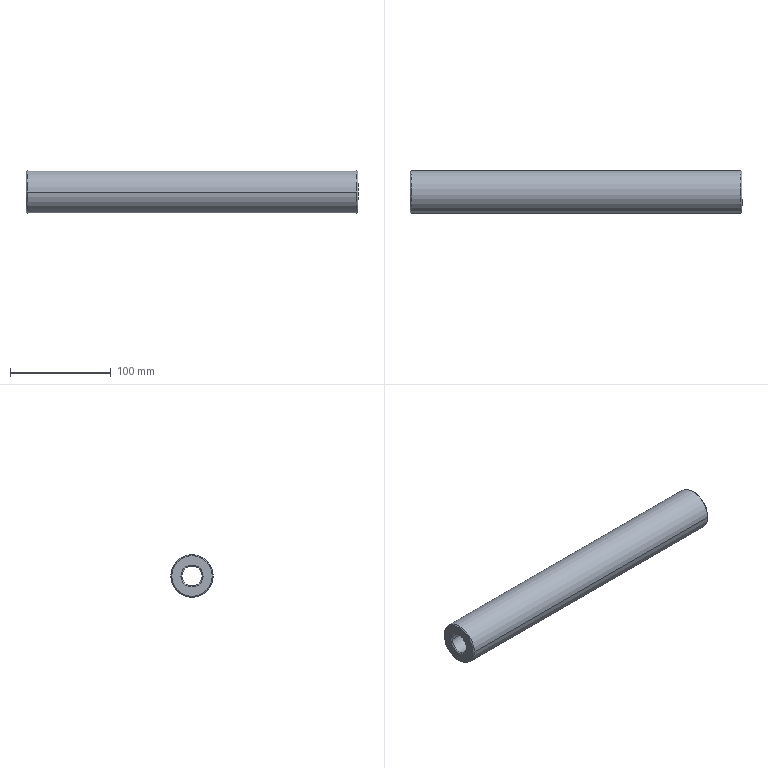Part | SolidWorks | features BaseBody 1 | 1 solid | 20 faces | box 330 x 42.2 x 42.2 mm | volume 188080 mm3 | cylinder 8 | cone 8 | plane 4 | commonest cylinder face diameters 20 x4 35.08 x2 42.2 x2
STEP:
#1=CARTESIAN_POINT('',(-40.109,46.064,0.));
#2=VERTEX_POINT('',#1);
#3=CARTESIAN_POINT('',(-40.109,3.864,0.));
#4=VERTEX_POINT('',#3);
#5=CARTESIAN_POINT('',(-40.109,24.964,0.));
#6=DIRECTION('',(1.,0.,0.));
#7=DIRECTION('',(0.,1.,0.));
#8=AXIS2_PLACEMENT_3D('',#5,#6,#7);
#9=CIRCLE('',#8,21.1);
#10=EDGE_CURVE('',#2,#4,#9,.T.);
#11=ORIENTED_EDGE('',*,*,#10,.T.);
#12=CARTESIAN_POINT('',(287.891,3.864,0.));
#13=VERTEX_POINT('',#12);
#14=CARTESIAN_POINT('',(123.891,3.864,0.));
#15=DIRECTION('',(1.,0.,0.));
#16=VECTOR('',#15,1000.);
#17=LINE('',#14,#16);
#18=EDGE_CURVE('',#4,#13,#17,.T.);
#19=ORIENTED_EDGE('',*,*,#18,.T.);
#20=CARTESIAN_POINT('',(287.891,46.064,0.));
#21=VERTEX_POINT('',#20);
#22=CARTESIAN_POINT('',(287.891,24.964,0.));
#23=DIRECTION('',(-1.,0.,0.));
#24=DIRECTION('',(0.,1.,0.));
#25=AXIS2_PLACEMENT_3D('',#22,#23,#24);
#26=CIRCLE('',#25,21.1);
#27=EDGE_CURVE('',#13,#21,#26,.T.);
#28=ORIENTED_EDGE('',*,*,#27,.T.);
#29=CARTESIAN_POINT('',(123.891,46.064,0.));
#30=DIRECTION('',(1.,0.,0.));
#31=VECTOR('',#30,1000.);
#32=LINE('',#29,#31);
#33=EDGE_CURVE('',#2,#21,#32,.T.);
#34=ORIENTED_EDGE('',*,*,#33,.F.);
#35=EDGE_LOOP('',(#11,#19,#28,#34));
#36=FACE_OUTER_BOUND('',#35,.T.);
#37=CARTESIAN_POINT('',(123.891,24.964,0.));
#38=DIRECTION('',(1.,0.,0.));
#39=DIRECTION('',(0.,1.,0.));
#40=AXIS2_PLACEMENT_3D('',#37,#38,#39);
#41=CYLINDRICAL_SURFACE('',#40,21.1);
#42=ADVANCED_FACE('',(#36),#41,.T.);
#43=CARTESIAN_POINT('',(288.891,4.864,0.));
#44=VERTEX_POINT('',#43);
#45=CARTESIAN_POINT('',(288.891,45.064,0.));
#46=VERTEX_POINT('',#45);
#47=CARTESIAN_POINT('',(288.891,24.964,0.));
#48=DIRECTION('',(-1.,0.,0.));
#49=DIRECTION('',(0.,-1.,0.));
#50=AXIS2_PLACEMENT_3D('',#47,#48,#49);
#51=CIRCLE('',#50,20.1);
#52=EDGE_CURVE('',#44,#46,#51,.T.);
#53=ORIENTED_EDGE('',*,*,#52,.T.);
#54=CARTESIAN_POINT('',(287.891,46.064,0.));
#55=DIRECTION('',(-0.7071,0.7071,0.));
#56=VECTOR('',#55,1000.);
#57=LINE('',#54,#56);
#58=EDGE_CURVE('',#46,#21,#57,.T.);
#59=ORIENTED_EDGE('',*,*,#58,.T.);
#60=ORIENTED_EDGE('',*,*,#27,.F.);
#61=CARTESIAN_POINT('',(287.891,3.864,0.));
#62=DIRECTION('',(-0.7071,-0.7071,0.));
#63=VECTOR('',#62,1000.);
#64=LINE('',#61,#63);
#65=EDGE_CURVE('',#44,#13,#64,.T.);
#66=ORIENTED_EDGE('',*,*,#65,.F.);
#67=EDGE_LOOP('',(#53,#59,#60,#66));
#68=FACE_OUTER_BOUND('',#67,.T.);
#69=CARTESIAN_POINT('',(287.891,24.964,0.));
#70=DIRECTION('',(-1.,0.,0.));
#71=DIRECTION('',(0.,-1.,0.));
#72=AXIS2_PLACEMENT_3D('',#69,#70,#71);
#73=CONICAL_SURFACE('',#72,21.1,0.7854);
#74=ADVANCED_FACE('',(#68),#73,.T.);
#75=CARTESIAN_POINT('',(-41.109,45.064,0.));
#76=VERTEX_POINT('',#75);
#77=CARTESIAN_POINT('',(-41.109,4.864,0.));
#78=VERTEX_POINT('',#77);
#79=CARTESIAN_POINT('',(-41.109,24.964,0.));
#80=DIRECTION('',(1.,0.,0.));
#81=DIRECTION('',(0.,1.,0.));
#82=AXIS2_PLACEMENT_3D('',#79,#80,#81);
#83=CIRCLE('',#82,20.1);
#84=EDGE_CURVE('',#76,#78,#83,.T.);
#85=ORIENTED_EDGE('',*,*,#84,.T.);
#86=CARTESIAN_POINT('',(-40.109,3.864,0.));
#87=DIRECTION('',(0.7071,-0.7071,0.));
#88=VECTOR('',#87,1000.);
#89=LINE('',#86,#88);
#90=EDGE_CURVE('',#78,#4,#89,.T.);
#91=ORIENTED_EDGE('',*,*,#90,.T.);
#92=ORIENTED_EDGE('',*,*,#10,.F.);
#93=CARTESIAN_POINT('',(-40.109,46.064,0.));
#94=DIRECTION('',(0.7071,0.7071,0.));
#95=VECTOR('',#94,1000.);
#96=LINE('',#93,#95);
#97=EDGE_CURVE('',#76,#2,#96,.T.);
#98=ORIENTED_EDGE('',*,*,#97,.F.);
#99=EDGE_LOOP('',(#85,#91,#92,#98));
#100=FACE_OUTER_BOUND('',#99,.T.);
#101=CARTESIAN_POINT('',(-40.109,24.964,0.));
#102=DIRECTION('',(1.,0.,0.));
#103=DIRECTION('',(0.,1.,0.));
#104=AXIS2_PLACEMENT_3D('',#101,#102,#103);
#105=CONICAL_SURFACE('',#104,21.1,0.7854);
#106=ADVANCED_FACE('',(#100),#105,.T.);
#107=CARTESIAN_POINT('',(287.891,14.964,0.));
#108=VERTEX_POINT('',#107);
#109=CARTESIAN_POINT('',(287.891,34.964,0.));
#110=VERTEX_POINT('',#109);
#111=CARTESIAN_POINT('',(287.891,24.964,0.));
#112=DIRECTION('',(1.,0.,0.));
#113=DIRECTION('',(0.,-1.,0.));
#114=AXIS2_PLACEMENT_3D('',#111,#112,#113);
#115=CIRCLE('',#114,10.);
#116=EDGE_CURVE('',#108,#110,#115,.T.);
#117=ORIENTED_EDGE('',*,*,#116,.F.);
#118=CARTESIAN_POINT('',(288.891,13.964,0.));
#119=VERTEX_POINT('',#118);
#120=CARTESIAN_POINT('',(288.891,13.964,0.));
#121=DIRECTION('',(0.7071,-0.7071,0.));
#122=VECTOR('',#121,1000.);
#123=LINE('',#120,#122);
#124=EDGE_CURVE('',#108,#119,#123,.T.);
#125=ORIENTED_EDGE('',*,*,#124,.T.);
#126=CARTESIAN_POINT('',(288.891,35.964,0.));
#127=VERTEX_POINT('',#126);
#128=CARTESIAN_POINT('',(288.891,24.964,0.));
#129=DIRECTION('',(-1.,0.,0.));
#130=DIRECTION('',(0.,1.,0.));
#131=AXIS2_PLACEMENT_3D('',#128,#129,#130);
#132=CIRCLE('',#131,11.);
#133=EDGE_CURVE('',#127,#119,#132,.T.);
#134=ORIENTED_EDGE('',*,*,#133,.F.);
#135=CARTESIAN_POINT('',(288.891,35.964,0.));
#136=DIRECTION('',(0.7071,0.7071,0.));
#137=VECTOR('',#136,1000.);
#138=LINE('',#135,#137);
#139=EDGE_CURVE('',#110,#127,#138,.T.);
#140=ORIENTED_EDGE('',*,*,#139,.F.);
#141=EDGE_LOOP('',(#117,#125,#134,#140));
#142=FACE_OUTER_BOUND('',#141,.T.);
#143=CARTESIAN_POINT('',(288.891,24.964,0.));
#144=DIRECTION('',(1.,0.,0.));
#145=DIRECTION('',(0.,1.,0.));
#146=AXIS2_PLACEMENT_3D('',#143,#144,#145);
#147=CONICAL_SURFACE('',#146,11.,0.7854);
#148=ADVANCED_FACE('',(#142),#147,.F.);
#149=CARTESIAN_POINT('',(-40.109,34.964,0.));
#150=VERTEX_POINT('',#149);
#151=CARTESIAN_POINT('',(-40.109,14.964,0.));
#152=VERTEX_POINT('',#151);
#153=CARTESIAN_POINT('',(-40.109,24.964,0.));
#154=DIRECTION('',(-1.,0.,0.));
#155=DIRECTION('',(0.,-1.,0.));
#156=AXIS2_PLACEMENT_3D('',#153,#154,#155);
#157=CIRCLE('',#156,10.);
#158=EDGE_CURVE('',#150,#152,#157,.T.);
#159=ORIENTED_EDGE('',*,*,#158,.F.);
#160=CARTESIAN_POINT('',(-41.109,35.964,0.));
#161=VERTEX_POINT('',#160);
#162=CARTESIAN_POINT('',(-41.109,35.964,0.));
#163=DIRECTION('',(-0.7071,0.7071,0.));
#164=VECTOR('',#163,1000.);
#165=LINE('',#162,#164);
#166=EDGE_CURVE('',#150,#161,#165,.T.);
#167=ORIENTED_EDGE('',*,*,#166,.T.);
#168=CARTESIAN_POINT('',(-41.109,13.964,0.));
#169=VERTEX_POINT('',#168);
#170=CARTESIAN_POINT('',(-41.109,24.964,0.));
#171=DIRECTION('',(1.,0.,0.));
#172=DIRECTION('',(0.,-1.,0.));
#173=AXIS2_PLACEMENT_3D('',#170,#171,#172);
#174=CIRCLE('',#173,11.);
#175=EDGE_CURVE('',#169,#161,#174,.T.);
#176=ORIENTED_EDGE('',*,*,#175,.F.);
#177=CARTESIAN_POINT('',(-41.109,13.964,0.));
#178=DIRECTION('',(-0.7071,-0.7071,0.));
#179=VECTOR('',#178,1000.);
#180=LINE('',#177,#179);
#181=EDGE_CURVE('',#152,#169,#180,.T.);
#182=ORIENTED_EDGE('',*,*,#181,.F.);
#183=EDGE_LOOP('',(#159,#167,#176,#182));
#184=FACE_OUTER_BOUND('',#183,.T.);
#185=CARTESIAN_POINT('',(-41.109,24.964,0.));
#186=DIRECTION('',(-1.,0.,0.));
#187=DIRECTION('',(0.,-1.,0.));
#188=AXIS2_PLACEMENT_3D('',#185,#186,#187);
#189=CONICAL_SURFACE('',#188,11.,0.7854);
#190=ADVANCED_FACE('',(#184),#189,.F.);
#191=CARTESIAN_POINT('',(253.891,14.964,0.));
#192=VERTEX_POINT('',#191);
#193=CARTESIAN_POINT('',(253.891,34.964,0.));
#194=VERTEX_POINT('',#193);
#195=CARTESIAN_POINT('',(253.891,24.964,0.));
#196=DIRECTION('',(1.,0.,0.));
#197=DIRECTION('',(0.,1.,0.));
#198=AXIS2_PLACEMENT_3D('',#195,#196,#197);
#199=CIRCLE('',#198,10.);
#200=EDGE_CURVE('',#192,#194,#199,.T.);
#201=ORIENTED_EDGE('',*,*,#200,.F.);
#202=CARTESIAN_POINT('',(271.391,14.964,0.));
#203=DIRECTION('',(1.,0.,0.));
#204=VECTOR('',#203,1000.);
#205=LINE('',#202,#204);
#206=EDGE_CURVE('',#192,#108,#205,.T.);
#207=ORIENTED_EDGE('',*,*,#206,.T.);
#208=ORIENTED_EDGE('',*,*,#116,.T.);
#209=CARTESIAN_POINT('',(271.391,34.964,0.));
#210=DIRECTION('',(1.,0.,0.));
#211=VECTOR('',#210,1000.);
#212=LINE('',#209,#211);
#213=EDGE_CURVE('',#194,#110,#212,.T.);
#214=ORIENTED_EDGE('',*,*,#213,.F.);
#215=EDGE_LOOP('',(#201,#207,#208,#214));
#216=FACE_OUTER_BOUND('',#215,.T.);
#217=CARTESIAN_POINT('',(271.391,24.964,0.));
#218=DIRECTION('',(1.,0.,0.));
#219=DIRECTION('',(0.,1.,0.));
#220=AXIS2_PLACEMENT_3D('',#217,#218,#219);
#221=CYLINDRICAL_SURFACE('',#220,10.);
#222=ADVANCED_FACE('',(#216),#221,.F.);
#223=ORIENTED_EDGE('',*,*,#158,.T.);
#224=CARTESIAN_POINT('',(-6.109,14.964,0.));
#225=VERTEX_POINT('',#224);
#226=CARTESIAN_POINT('',(-23.609,14.964,0.));
#227=DIRECTION('',(1.,0.,0.));
#228=VECTOR('',#227,1000.);
#229=LINE('',#226,#228);
#230=EDGE_CURVE('',#152,#225,#229,.T.);
#231=ORIENTED_EDGE('',*,*,#230,.T.);
#232=CARTESIAN_POINT('',(-6.109,34.964,0.));
#233=VERTEX_POINT('',#232);
#234=CARTESIAN_POINT('',(-6.109,24.964,0.));
#235=DIRECTION('',(-1.,0.,0.));
#236=DIRECTION('',(0.,1.,0.));
#237=AXIS2_PLACEMENT_3D('',#234,#235,#236);
#238=CIRCLE('',#237,10.);
#239=EDGE_CURVE('',#233,#225,#238,.T.);
#240=ORIENTED_EDGE('',*,*,#239,.F.);
#241=CARTESIAN_POINT('',(-23.609,34.964,0.));
#242=DIRECTION('',(1.,0.,0.));
#243=VECTOR('',#242,1000.);
#244=LINE('',#241,#243);
#245=EDGE_CURVE('',#150,#233,#244,.T.);
#246=ORIENTED_EDGE('',*,*,#245,.F.);
#247=EDGE_LOOP('',(#223,#231,#240,#246));
#248=FACE_OUTER_BOUND('',#247,.T.);
#249=CARTESIAN_POINT('',(-23.609,24.964,0.));
#250=DIRECTION('',(1.,0.,0.));
#251=DIRECTION('',(0.,1.,0.));
#252=AXIS2_PLACEMENT_3D('',#249,#250,#251);
#253=CYLINDRICAL_SURFACE('',#252,10.);
#254=ADVANCED_FACE('',(#248),#253,.F.);
#255=CARTESIAN_POINT('',(-6.109,7.424,0.));
#256=VERTEX_POINT('',#255);
#257=CARTESIAN_POINT('',(-6.109,42.504,0.));
#258=VERTEX_POINT('',#257);
#259=CARTESIAN_POINT('',(-6.109,24.964,0.));
#260=DIRECTION('',(1.,0.,0.));
#261=DIRECTION('',(0.,1.,0.));
#262=AXIS2_PLACEMENT_3D('',#259,#260,#261);
#263=CIRCLE('',#262,17.54);
#264=EDGE_CURVE('',#256,#258,#263,.T.);
#265=ORIENTED_EDGE('',*,*,#264,.F.);
#266=CARTESIAN_POINT('',(253.891,7.424,0.));
#267=VERTEX_POINT('',#266);
#268=CARTESIAN_POINT('',(123.891,7.424,0.));
#269=DIRECTION('',(1.,0.,0.));
#270=VECTOR('',#269,1000.);
#271=LINE('',#268,#270);
#272=EDGE_CURVE('',#256,#267,#271,.T.);
#273=ORIENTED_EDGE('',*,*,#272,.T.);
#274=CARTESIAN_POINT('',(253.891,42.504,0.));
#275=VERTEX_POINT('',#274);
#276=CARTESIAN_POINT('',(253.891,24.964,0.));
#277=DIRECTION('',(-1.,0.,0.));
#278=DIRECTION('',(0.,1.,0.));
#279=AXIS2_PLACEMENT_3D('',#276,#277,#278);
#280=CIRCLE('',#279,17.54);
#281=EDGE_CURVE('',#275,#267,#280,.T.);
#282=ORIENTED_EDGE('',*,*,#281,.F.);
#283=CARTESIAN_POINT('',(123.891,42.504,0.));
#284=DIRECTION('',(1.,0.,0.));
#285=VECTOR('',#284,1000.);
#286=LINE('',#283,#285);
#287=EDGE_CURVE('',#258,#275,#286,.T.);
#288=ORIENTED_EDGE('',*,*,#287,.F.);
#289=EDGE_LOOP('',(#265,#273,#282,#288));
#290=FACE_OUTER_BOUND('',#289,.T.);
#291=CARTESIAN_POINT('',(123.891,24.964,0.));
#292=DIRECTION('',(1.,0.,0.));
#293=DIRECTION('',(0.,1.,0.));
#294=AXIS2_PLACEMENT_3D('',#291,#292,#293);
#295=CYLINDRICAL_SURFACE('',#294,17.54);
#296=ADVANCED_FACE('',(#290),#295,.F.);
#297=ORIENTED_EDGE('',*,*,#18,.F.);
#298=CARTESIAN_POINT('',(-40.109,24.964,0.));
#299=DIRECTION('',(1.,0.,0.));
#300=DIRECTION('',(0.,1.,0.));
#301=AXIS2_PLACEMENT_3D('',#298,#299,#300);
#302=CIRCLE('',#301,21.1);
#303=EDGE_CURVE('',#4,#2,#302,.T.);
#304=ORIENTED_EDGE('',*,*,#303,.T.);
#305=ORIENTED_EDGE('',*,*,#33,.T.);
#306=CARTESIAN_POINT('',(287.891,24.964,0.));
#307=DIRECTION('',(-1.,0.,0.));
#308=DIRECTION('',(0.,1.,0.));
#309=AXIS2_PLACEMENT_3D('',#306,#307,#308);
#310=CIRCLE('',#309,21.1);
#311=EDGE_CURVE('',#21,#13,#310,.T.);
#312=ORIENTED_EDGE('',*,*,#311,.T.);
#313=EDGE_LOOP('',(#297,#304,#305,#312));
#314=FACE_OUTER_BOUND('',#313,.T.);
#315=CARTESIAN_POINT('',(123.891,24.964,0.));
#316=DIRECTION('',(1.,0.,0.));
#317=DIRECTION('',(0.,1.,0.));
#318=AXIS2_PLACEMENT_3D('',#315,#316,#317);
#319=CYLINDRICAL_SURFACE('',#318,21.1);
#320=ADVANCED_FACE('',(#314),#319,.T.);
#321=ORIENTED_EDGE('',*,*,#58,.F.);
#322=CARTESIAN_POINT('',(288.891,24.964,0.));
#323=DIRECTION('',(-1.,0.,0.));
#324=DIRECTION('',(0.,-1.,0.));
#325=AXIS2_PLACEMENT_3D('',#322,#323,#324);
#326=CIRCLE('',#325,20.1);
#327=EDGE_CURVE('',#46,#44,#326,.T.);
#328=ORIENTED_EDGE('',*,*,#327,.T.);
#329=ORIENTED_EDGE('',*,*,#65,.T.);
#330=ORIENTED_EDGE('',*,*,#311,.F.);
#331=EDGE_LOOP('',(#321,#328,#329,#330));
#332=FACE_OUTER_BOUND('',#331,.T.);
#333=CARTESIAN_POINT('',(287.891,24.964,0.));
#334=DIRECTION('',(-1.,0.,0.));
#335=DIRECTION('',(0.,-1.,0.));
#336=AXIS2_PLACEMENT_3D('',#333,#334,#335);
#337=CONICAL_SURFACE('',#336,21.1,0.7854);
#338=ADVANCED_FACE('',(#332),#337,.T.);
#339=ORIENTED_EDGE('',*,*,#90,.F.);
#340=CARTESIAN_POINT('',(-41.109,24.964,0.));
#341=DIRECTION('',(1.,0.,0.));
#342=DIRECTION('',(0.,1.,0.));
#343=AXIS2_PLACEMENT_3D('',#340,#341,#342);
#344=CIRCLE('',#343,20.1);
#345=EDGE_CURVE('',#78,#76,#344,.T.);
#346=ORIENTED_EDGE('',*,*,#345,.T.);
#347=ORIENTED_EDGE('',*,*,#97,.T.);
#348=ORIENTED_EDGE('',*,*,#303,.F.);
#349=EDGE_LOOP('',(#339,#346,#347,#348));
#350=FACE_OUTER_BOUND('',#349,.T.);
#351=CARTESIAN_POINT('',(-40.109,24.964,0.));
#352=DIRECTION('',(1.,0.,0.));
#353=DIRECTION('',(0.,1.,0.));
#354=AXIS2_PLACEMENT_3D('',#351,#352,#353);
#355=CONICAL_SURFACE('',#354,21.1,0.7854);
#356=ADVANCED_FACE('',(#350),#355,.T.);
#357=ORIENTED_EDGE('',*,*,#133,.T.);
#358=CARTESIAN_POINT('',(288.891,24.964,0.));
#359=DIRECTION('',(-1.,0.,0.));
#360=DIRECTION('',(0.,1.,0.));
#361=AXIS2_PLACEMENT_3D('',#358,#359,#360);
#362=CIRCLE('',#361,11.);
#363=EDGE_CURVE('',#119,#127,#362,.T.);
#364=ORIENTED_EDGE('',*,*,#363,.T.);
#365=EDGE_LOOP('',(#357,#364));
#366=FACE_BOUND('',#365,.T.);
#367=ORIENTED_EDGE('',*,*,#52,.F.);
#368=ORIENTED_EDGE('',*,*,#327,.F.);
#369=EDGE_LOOP('',(#367,#368));
#370=FACE_OUTER_BOUND('',#369,.T.);
#371=CARTESIAN_POINT('',(288.891,40.514,0.));
#372=DIRECTION('',(1.,0.,0.));
#373=DIRECTION('',(0.,1.,0.));
#374=AXIS2_PLACEMENT_3D('',#371,#372,#373);
#375=PLANE('',#374);
#376=ADVANCED_FACE('',(#366,#370),#375,.T.);
#377=ORIENTED_EDGE('',*,*,#175,.T.);
#378=CARTESIAN_POINT('',(-41.109,24.964,0.));
#379=DIRECTION('',(1.,0.,0.));
#380=DIRECTION('',(0.,-1.,0.));
#381=AXIS2_PLACEMENT_3D('',#378,#379,#380);
#382=CIRCLE('',#381,11.);
#383=EDGE_CURVE('',#161,#169,#382,.T.);
#384=ORIENTED_EDGE('',*,*,#383,.T.);
#385=EDGE_LOOP('',(#377,#384));
#386=FACE_BOUND('',#385,.T.);
#387=ORIENTED_EDGE('',*,*,#84,.F.);
#388=ORIENTED_EDGE('',*,*,#345,.F.);
#389=EDGE_LOOP('',(#387,#388));
#390=FACE_OUTER_BOUND('',#389,.T.);
#391=CARTESIAN_POINT('',(-41.109,40.514,0.));
#392=DIRECTION('',(-1.,0.,0.));
#393=DIRECTION('',(0.,-1.,0.));
#394=AXIS2_PLACEMENT_3D('',#391,#392,#393);
#395=PLANE('',#394);
#396=ADVANCED_FACE('',(#386,#390),#395,.T.);
#397=ORIENTED_EDGE('',*,*,#124,.F.);
#398=CARTESIAN_POINT('',(287.891,24.964,0.));
#399=DIRECTION('',(1.,0.,0.));
#400=DIRECTION('',(0.,-1.,0.));
#401=AXIS2_PLACEMENT_3D('',#398,#399,#400);
#402=CIRCLE('',#401,10.);
#403=EDGE_CURVE('',#110,#108,#402,.T.);
#404=ORIENTED_EDGE('',*,*,#403,.F.);
#405=ORIENTED_EDGE('',*,*,#139,.T.);
#406=ORIENTED_EDGE('',*,*,#363,.F.);
#407=EDGE_LOOP('',(#397,#404,#405,#406));
#408=FACE_OUTER_BOUND('',#407,.T.);
#409=CARTESIAN_POINT('',(288.891,24.964,0.));
#410=DIRECTION('',(1.,0.,0.));
#411=DIRECTION('',(0.,1.,0.));
#412=AXIS2_PLACEMENT_3D('',#409,#410,#411);
#413=CONICAL_SURFACE('',#412,11.,0.7854);
#414=ADVANCED_FACE('',(#408),#413,.F.);
#415=ORIENTED_EDGE('',*,*,#166,.F.);
#416=CARTESIAN_POINT('',(-40.109,24.964,0.));
#417=DIRECTION('',(-1.,0.,0.));
#418=DIRECTION('',(0.,-1.,0.));
#419=AXIS2_PLACEMENT_3D('',#416,#417,#418);
#420=CIRCLE('',#419,10.);
#421=EDGE_CURVE('',#152,#150,#420,.T.);
#422=ORIENTED_EDGE('',*,*,#421,.F.);
#423=ORIENTED_EDGE('',*,*,#181,.T.);
#424=ORIENTED_EDGE('',*,*,#383,.F.);
#425=EDGE_LOOP('',(#415,#422,#423,#424));
#426=FACE_OUTER_BOUND('',#425,.T.);
#427=CARTESIAN_POINT('',(-41.109,24.964,0.));
#428=DIRECTION('',(-1.,0.,0.));
#429=DIRECTION('',(0.,-1.,0.));
#430=AXIS2_PLACEMENT_3D('',#427,#428,#429);
#431=CONICAL_SURFACE('',#430,11.,0.7854);
#432=ADVANCED_FACE('',(#426),#431,.F.);
#433=ORIENTED_EDGE('',*,*,#206,.F.);
#434=CARTESIAN_POINT('',(253.891,24.964,0.));
#435=DIRECTION('',(1.,0.,0.));
#436=DIRECTION('',(0.,1.,0.));
#437=AXIS2_PLACEMENT_3D('',#434,#435,#436);
#438=CIRCLE('',#437,10.);
#439=EDGE_CURVE('',#194,#192,#438,.T.);
#440=ORIENTED_EDGE('',*,*,#439,.F.);
#441=ORIENTED_EDGE('',*,*,#213,.T.);
#442=ORIENTED_EDGE('',*,*,#403,.T.);
#443=EDGE_LOOP('',(#433,#440,#441,#442));
#444=FACE_OUTER_BOUND('',#443,.T.);
#445=CARTESIAN_POINT('',(271.391,24.964,0.));
#446=DIRECTION('',(1.,0.,0.));
#447=DIRECTION('',(0.,1.,0.));
#448=AXIS2_PLACEMENT_3D('',#445,#446,#447);
#449=CYLINDRICAL_SURFACE('',#448,10.);
#450=ADVANCED_FACE('',(#444),#449,.F.);
#451=ORIENTED_EDGE('',*,*,#230,.F.);
#452=ORIENTED_EDGE('',*,*,#421,.T.);
#453=ORIENTED_EDGE('',*,*,#245,.T.);
#454=CARTESIAN_POINT('',(-6.109,24.964,0.));
#455=DIRECTION('',(-1.,0.,0.));
#456=DIRECTION('',(0.,1.,0.));
#457=AXIS2_PLACEMENT_3D('',#454,#455,#456);
#458=CIRCLE('',#457,10.);
#459=EDGE_CURVE('',#225,#233,#458,.T.);
#460=ORIENTED_EDGE('',*,*,#459,.F.);
#461=EDGE_LOOP('',(#451,#452,#453,#460));
#462=FACE_OUTER_BOUND('',#461,.T.);
#463=CARTESIAN_POINT('',(-23.609,24.964,0.));
#464=DIRECTION('',(1.,0.,0.));
#465=DIRECTION('',(0.,1.,0.));
#466=AXIS2_PLACEMENT_3D('',#463,#464,#465);
#467=CYLINDRICAL_SURFACE('',#466,10.);
#468=ADVANCED_FACE('',(#462),#467,.F.);
#469=ORIENTED_EDGE('',*,*,#439,.T.);
#470=ORIENTED_EDGE('',*,*,#200,.T.);
#471=EDGE_LOOP('',(#469,#470));
#472=FACE_BOUND('',#471,.T.);
#473=ORIENTED_EDGE('',*,*,#281,.T.);
#474=CARTESIAN_POINT('',(253.891,24.964,0.));
#475=DIRECTION('',(-1.,0.,0.));
#476=DIRECTION('',(0.,1.,0.));
#477=AXIS2_PLACEMENT_3D('',#474,#475,#476);
#478=CIRCLE('',#477,17.54);
#479=EDGE_CURVE('',#267,#275,#478,.T.);
#480=ORIENTED_EDGE('',*,*,#479,.T.);
#481=EDGE_LOOP('',(#473,#480));
#482=FACE_OUTER_BOUND('',#481,.T.);
#483=CARTESIAN_POINT('',(253.891,38.734,0.));
#484=DIRECTION('',(-1.,0.,0.));
#485=DIRECTION('',(0.,-1.,0.));
#486=AXIS2_PLACEMENT_3D('',#483,#484,#485);
#487=PLANE('',#486);
#488=ADVANCED_FACE('',(#472,#482),#487,.T.);
#489=ORIENTED_EDGE('',*,*,#239,.T.);
#490=ORIENTED_EDGE('',*,*,#459,.T.);
#491=EDGE_LOOP('',(#489,#490));
#492=FACE_BOUND('',#491,.T.);
#493=CARTESIAN_POINT('',(-6.109,24.964,0.));
#494=DIRECTION('',(1.,0.,0.));
#495=DIRECTION('',(0.,1.,0.));
#496=AXIS2_PLACEMENT_3D('',#493,#494,#495);
#497=CIRCLE('',#496,17.54);
#498=EDGE_CURVE('',#258,#256,#497,.T.);
#499=ORIENTED_EDGE('',*,*,#498,.T.);
#500=ORIENTED_EDGE('',*,*,#264,.T.);
#501=EDGE_LOOP('',(#499,#500));
#502=FACE_OUTER_BOUND('',#501,.T.);
#503=CARTESIAN_POINT('',(-6.109,38.734,0.));
#504=DIRECTION('',(1.,0.,0.));
#505=DIRECTION('',(0.,1.,0.));
#506=AXIS2_PLACEMENT_3D('',#503,#504,#505);
#507=PLANE('',#506);
#508=ADVANCED_FACE('',(#492,#502),#507,.T.);
#509=ORIENTED_EDGE('',*,*,#272,.F.);
#510=ORIENTED_EDGE('',*,*,#498,.F.);
#511=ORIENTED_EDGE('',*,*,#287,.T.);
#512=ORIENTED_EDGE('',*,*,#479,.F.);
#513=EDGE_LOOP('',(#509,#510,#511,#512));
#514=FACE_OUTER_BOUND('',#513,.T.);
#515=CARTESIAN_POINT('',(123.891,24.964,0.));
#516=DIRECTION('',(1.,0.,0.));
#517=DIRECTION('',(0.,1.,0.));
#518=AXIS2_PLACEMENT_3D('',#515,#516,#517);
#519=CYLINDRICAL_SURFACE('',#518,17.54);
#520=ADVANCED_FACE('',(#514),#519,.F.);
#521=CLOSED_SHELL('',(#42,#74,#106,#148,#190,#222,#254,#296,#320,#338,#356,#376,#396,#414,#432,#450,#468,#488,#508,#520));
#522=MANIFOLD_SOLID_BREP('',#521);
#523=CARTESIAN_POINT('',(0.,0.,0.));
#524=DIRECTION('',(0.,0.,1.));
#525=DIRECTION('',(1.,0.,0.));
#526=AXIS2_PLACEMENT_3D('',#523,#524,#525);
#527=(LENGTH_UNIT()NAMED_UNIT(*)SI_UNIT(.MILLI.,.METRE.));
#528=UNCERTAINTY_MEASURE_WITH_UNIT(LENGTH_MEASURE(0.00001),#527,'','');
#529=(NAMED_UNIT(*)PLANE_ANGLE_UNIT()SI_UNIT($,.RADIAN.));
#530=(NAMED_UNIT(*)SI_UNIT($,.STERADIAN.)SOLID_ANGLE_UNIT());
#531=(GEOMETRIC_REPRESENTATION_CONTEXT(3)GLOBAL_UNCERTAINTY_ASSIGNED_CONTEXT((#528))GLOBAL_UNIT_ASSIGNED_CONTEXT((#527,#529,#530))REPRESENTATION_CONTEXT('',''));
#532=ADVANCED_BREP_SHAPE_REPRESENTATION('',(#522,#526),#531);